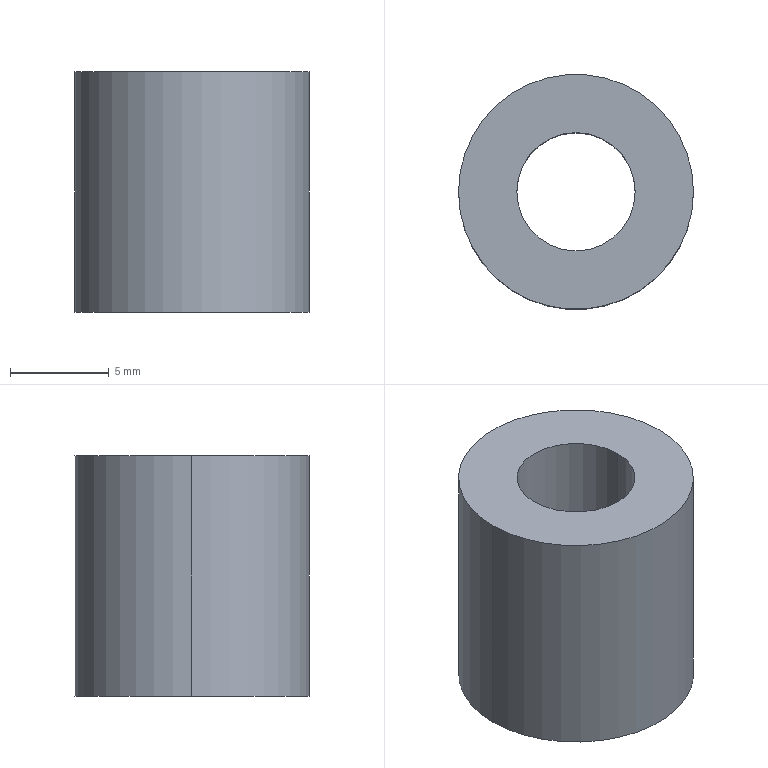Part | SolidWorks | features Extrusion 1 | 1 solid | 6 faces | box 11.91 x 11.91 x 12.2 mm | volume 1014 mm3 | cylinder 4 | plane 2 | commonest cylinder face diameters 6 x2 11.91 x2
STEP:
#1=CARTESIAN_POINT('',(-3.,0.,12.2));
#2=VERTEX_POINT('',#1);
#3=CARTESIAN_POINT('',(3.,0.,12.2));
#4=VERTEX_POINT('',#3);
#5=CARTESIAN_POINT('',(0.,0.,12.2));
#6=DIRECTION('',(0.,0.,1.));
#7=DIRECTION('',(1.,0.,0.));
#8=AXIS2_PLACEMENT_3D('',#5,#6,#7);
#9=CIRCLE('',#8,3.);
#10=EDGE_CURVE('',#2,#4,#9,.T.);
#11=ORIENTED_EDGE('',*,*,#10,.T.);
#12=CARTESIAN_POINT('',(3.,0.,0.));
#13=VERTEX_POINT('',#12);
#14=CARTESIAN_POINT('',(3.,0.,12.2));
#15=DIRECTION('',(0.,0.,-1.));
#16=VECTOR('',#15,1000.);
#17=LINE('',#14,#16);
#18=EDGE_CURVE('',#4,#13,#17,.T.);
#19=ORIENTED_EDGE('',*,*,#18,.T.);
#20=CARTESIAN_POINT('',(-3.,0.,0.));
#21=VERTEX_POINT('',#20);
#22=CARTESIAN_POINT('',(0.,0.,0.));
#23=DIRECTION('',(0.,0.,1.));
#24=DIRECTION('',(1.,0.,0.));
#25=AXIS2_PLACEMENT_3D('',#22,#23,#24);
#26=CIRCLE('',#25,3.);
#27=EDGE_CURVE('',#21,#13,#26,.T.);
#28=ORIENTED_EDGE('',*,*,#27,.F.);
#29=CARTESIAN_POINT('',(-3.,0.,12.2));
#30=DIRECTION('',(0.,0.,-1.));
#31=VECTOR('',#30,1000.);
#32=LINE('',#29,#31);
#33=EDGE_CURVE('',#2,#21,#32,.T.);
#34=ORIENTED_EDGE('',*,*,#33,.F.);
#35=EDGE_LOOP('',(#11,#19,#28,#34));
#36=FACE_OUTER_BOUND('',#35,.T.);
#37=CARTESIAN_POINT('',(0.,0.,12.2));
#38=DIRECTION('',(0.,0.,-1.));
#39=DIRECTION('',(-1.,0.,0.));
#40=AXIS2_PLACEMENT_3D('',#37,#38,#39);
#41=CYLINDRICAL_SURFACE('',#40,3.);
#42=ADVANCED_FACE('',(#36),#41,.F.);
#43=CARTESIAN_POINT('',(5.955,0.,12.2));
#44=VERTEX_POINT('',#43);
#45=CARTESIAN_POINT('',(-5.955,0.,12.2));
#46=VERTEX_POINT('',#45);
#47=CARTESIAN_POINT('',(0.,0.,12.2));
#48=DIRECTION('',(0.,0.,1.));
#49=DIRECTION('',(1.,0.,0.));
#50=AXIS2_PLACEMENT_3D('',#47,#48,#49);
#51=CIRCLE('',#50,5.955);
#52=EDGE_CURVE('',#44,#46,#51,.T.);
#53=ORIENTED_EDGE('',*,*,#52,.F.);
#54=CARTESIAN_POINT('',(5.955,0.,0.));
#55=VERTEX_POINT('',#54);
#56=CARTESIAN_POINT('',(5.955,0.,12.2));
#57=DIRECTION('',(0.,0.,-1.));
#58=VECTOR('',#57,1000.);
#59=LINE('',#56,#58);
#60=EDGE_CURVE('',#44,#55,#59,.T.);
#61=ORIENTED_EDGE('',*,*,#60,.T.);
#62=CARTESIAN_POINT('',(-5.955,0.,0.));
#63=VERTEX_POINT('',#62);
#64=CARTESIAN_POINT('',(0.,0.,0.));
#65=DIRECTION('',(0.,0.,1.));
#66=DIRECTION('',(1.,0.,0.));
#67=AXIS2_PLACEMENT_3D('',#64,#65,#66);
#68=CIRCLE('',#67,5.955);
#69=EDGE_CURVE('',#55,#63,#68,.T.);
#70=ORIENTED_EDGE('',*,*,#69,.T.);
#71=CARTESIAN_POINT('',(-5.955,0.,12.2));
#72=DIRECTION('',(0.,0.,-1.));
#73=VECTOR('',#72,1000.);
#74=LINE('',#71,#73);
#75=EDGE_CURVE('',#46,#63,#74,.T.);
#76=ORIENTED_EDGE('',*,*,#75,.F.);
#77=EDGE_LOOP('',(#53,#61,#70,#76));
#78=FACE_OUTER_BOUND('',#77,.T.);
#79=CARTESIAN_POINT('',(0.,0.,12.2));
#80=DIRECTION('',(0.,0.,-1.));
#81=DIRECTION('',(-1.,0.,0.));
#82=AXIS2_PLACEMENT_3D('',#79,#80,#81);
#83=CYLINDRICAL_SURFACE('',#82,5.955);
#84=ADVANCED_FACE('',(#78),#83,.T.);
#85=CARTESIAN_POINT('',(0.,0.,12.2));
#86=DIRECTION('',(0.,0.,1.));
#87=DIRECTION('',(1.,0.,0.));
#88=AXIS2_PLACEMENT_3D('',#85,#86,#87);
#89=CIRCLE('',#88,5.955);
#90=EDGE_CURVE('',#46,#44,#89,.T.);
#91=ORIENTED_EDGE('',*,*,#90,.T.);
#92=ORIENTED_EDGE('',*,*,#52,.T.);
#93=EDGE_LOOP('',(#91,#92));
#94=FACE_OUTER_BOUND('',#93,.T.);
#95=ORIENTED_EDGE('',*,*,#10,.F.);
#96=CARTESIAN_POINT('',(0.,0.,12.2));
#97=DIRECTION('',(0.,0.,1.));
#98=DIRECTION('',(1.,0.,0.));
#99=AXIS2_PLACEMENT_3D('',#96,#97,#98);
#100=CIRCLE('',#99,3.);
#101=EDGE_CURVE('',#4,#2,#100,.T.);
#102=ORIENTED_EDGE('',*,*,#101,.F.);
#103=EDGE_LOOP('',(#95,#102));
#104=FACE_BOUND('',#103,.T.);
#105=CARTESIAN_POINT('',(0.,0.,12.2));
#106=DIRECTION('',(0.,0.,1.));
#107=DIRECTION('',(1.,0.,0.));
#108=AXIS2_PLACEMENT_3D('',#105,#106,#107);
#109=PLANE('',#108);
#110=ADVANCED_FACE('',(#94,#104),#109,.T.);
#111=CARTESIAN_POINT('',(0.,0.,0.));
#112=DIRECTION('',(0.,0.,1.));
#113=DIRECTION('',(1.,0.,0.));
#114=AXIS2_PLACEMENT_3D('',#111,#112,#113);
#115=CIRCLE('',#114,5.955);
#116=EDGE_CURVE('',#63,#55,#115,.T.);
#117=ORIENTED_EDGE('',*,*,#116,.F.);
#118=ORIENTED_EDGE('',*,*,#69,.F.);
#119=EDGE_LOOP('',(#117,#118));
#120=FACE_OUTER_BOUND('',#119,.T.);
#121=ORIENTED_EDGE('',*,*,#27,.T.);
#122=CARTESIAN_POINT('',(0.,0.,0.));
#123=DIRECTION('',(0.,0.,1.));
#124=DIRECTION('',(1.,0.,0.));
#125=AXIS2_PLACEMENT_3D('',#122,#123,#124);
#126=CIRCLE('',#125,3.);
#127=EDGE_CURVE('',#13,#21,#126,.T.);
#128=ORIENTED_EDGE('',*,*,#127,.T.);
#129=EDGE_LOOP('',(#121,#128));
#130=FACE_BOUND('',#129,.T.);
#131=CARTESIAN_POINT('',(0.,0.,0.));
#132=DIRECTION('',(0.,0.,1.));
#133=DIRECTION('',(1.,0.,0.));
#134=AXIS2_PLACEMENT_3D('',#131,#132,#133);
#135=PLANE('',#134);
#136=ADVANCED_FACE('',(#120,#130),#135,.F.);
#137=ORIENTED_EDGE('',*,*,#60,.F.);
#138=ORIENTED_EDGE('',*,*,#90,.F.);
#139=ORIENTED_EDGE('',*,*,#75,.T.);
#140=ORIENTED_EDGE('',*,*,#116,.T.);
#141=EDGE_LOOP('',(#137,#138,#139,#140));
#142=FACE_OUTER_BOUND('',#141,.T.);
#143=CARTESIAN_POINT('',(0.,0.,12.2));
#144=DIRECTION('',(0.,0.,-1.));
#145=DIRECTION('',(-1.,0.,0.));
#146=AXIS2_PLACEMENT_3D('',#143,#144,#145);
#147=CYLINDRICAL_SURFACE('',#146,5.955);
#148=ADVANCED_FACE('',(#142),#147,.T.);
#149=ORIENTED_EDGE('',*,*,#18,.F.);
#150=ORIENTED_EDGE('',*,*,#101,.T.);
#151=ORIENTED_EDGE('',*,*,#33,.T.);
#152=ORIENTED_EDGE('',*,*,#127,.F.);
#153=EDGE_LOOP('',(#149,#150,#151,#152));
#154=FACE_OUTER_BOUND('',#153,.T.);
#155=CARTESIAN_POINT('',(0.,0.,12.2));
#156=DIRECTION('',(0.,0.,-1.));
#157=DIRECTION('',(-1.,0.,0.));
#158=AXIS2_PLACEMENT_3D('',#155,#156,#157);
#159=CYLINDRICAL_SURFACE('',#158,3.);
#160=ADVANCED_FACE('',(#154),#159,.F.);
#161=CLOSED_SHELL('',(#42,#84,#110,#136,#148,#160));
#162=MANIFOLD_SOLID_BREP('',#161);
#163=CARTESIAN_POINT('',(0.,0.,0.));
#164=DIRECTION('',(0.,0.,1.));
#165=DIRECTION('',(1.,0.,0.));
#166=AXIS2_PLACEMENT_3D('',#163,#164,#165);
#167=(LENGTH_UNIT()NAMED_UNIT(*)SI_UNIT(.MILLI.,.METRE.));
#168=UNCERTAINTY_MEASURE_WITH_UNIT(LENGTH_MEASURE(0.00001),#167,'','');
#169=(NAMED_UNIT(*)PLANE_ANGLE_UNIT()SI_UNIT($,.RADIAN.));
#170=(NAMED_UNIT(*)SI_UNIT($,.STERADIAN.)SOLID_ANGLE_UNIT());
#171=(GEOMETRIC_REPRESENTATION_CONTEXT(3)GLOBAL_UNCERTAINTY_ASSIGNED_CONTEXT((#168))GLOBAL_UNIT_ASSIGNED_CONTEXT((#167,#169,#170))REPRESENTATION_CONTEXT('',''));
#172=ADVANCED_BREP_SHAPE_REPRESENTATION('',(#162,#166),#171);